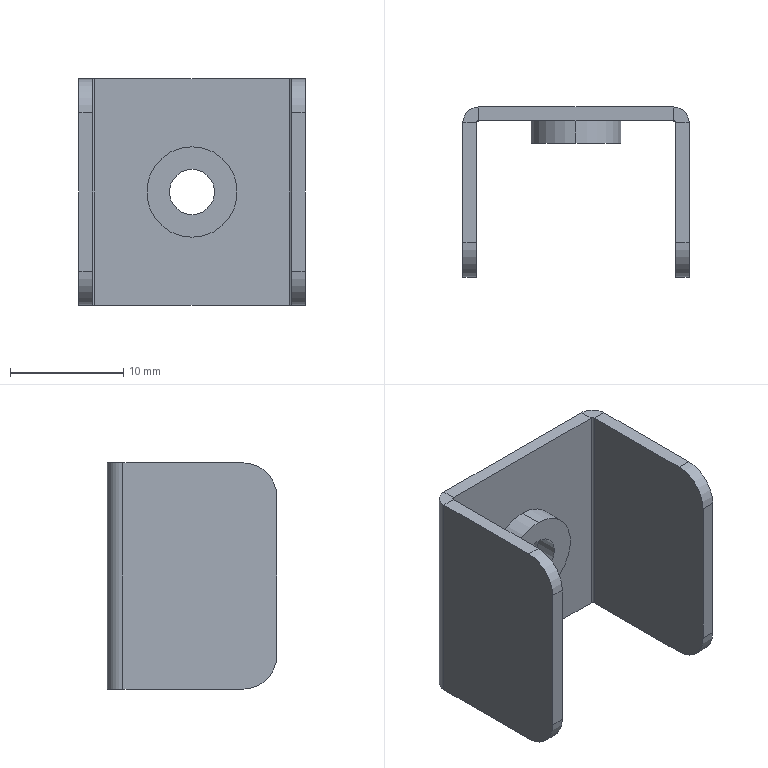Part | SolidWorks | features BaseBody 1 | 1 solid | 34 faces | box 20 x 15 x 20 mm | volume 1173 mm3 | plane 20 | cylinder 14 | commonest cylinder face diameters 6 x4 0.4 x2 2.8 x2 4 x2 4.5 x2 8 x2
STEP:
#1=CARTESIAN_POINT('',(0.,-3.2,-2.));
#2=VERTEX_POINT('',#1);
#3=CARTESIAN_POINT('',(0.,-1.2,-2.));
#4=VERTEX_POINT('',#3);
#5=CARTESIAN_POINT('',(0.,-3.2,-2.));
#6=DIRECTION('',(0.,1.,0.));
#7=VECTOR('',#6,1000.);
#8=LINE('',#5,#7);
#9=EDGE_CURVE('',#2,#4,#8,.T.);
#10=ORIENTED_EDGE('',*,*,#9,.F.);
#11=CARTESIAN_POINT('',(0.,-3.2,2.));
#12=VERTEX_POINT('',#11);
#13=CARTESIAN_POINT('',(0.,-3.2,0.));
#14=DIRECTION('',(0.,-1.,0.));
#15=DIRECTION('',(0.,0.,-1.));
#16=AXIS2_PLACEMENT_3D('',#13,#14,#15);
#17=CIRCLE('',#16,2.);
#18=EDGE_CURVE('',#2,#12,#17,.T.);
#19=ORIENTED_EDGE('',*,*,#18,.T.);
#20=CARTESIAN_POINT('',(0.,-1.2,2.));
#21=VERTEX_POINT('',#20);
#22=CARTESIAN_POINT('',(0.,-3.2,2.));
#23=DIRECTION('',(0.,1.,0.));
#24=VECTOR('',#23,1000.);
#25=LINE('',#22,#24);
#26=EDGE_CURVE('',#12,#21,#25,.T.);
#27=ORIENTED_EDGE('',*,*,#26,.T.);
#28=CARTESIAN_POINT('',(0.,-1.2,0.));
#29=DIRECTION('',(0.,-1.,0.));
#30=DIRECTION('',(0.,0.,-1.));
#31=AXIS2_PLACEMENT_3D('',#28,#29,#30);
#32=CIRCLE('',#31,2.);
#33=EDGE_CURVE('',#4,#21,#32,.T.);
#34=ORIENTED_EDGE('',*,*,#33,.F.);
#35=EDGE_LOOP('',(#10,#19,#27,#34));
#36=FACE_OUTER_BOUND('',#35,.T.);
#37=CARTESIAN_POINT('',(0.,-3.2,0.));
#38=DIRECTION('',(0.,1.,0.));
#39=DIRECTION('',(0.,0.,1.));
#40=AXIS2_PLACEMENT_3D('',#37,#38,#39);
#41=CYLINDRICAL_SURFACE('',#40,2.);
#42=ADVANCED_FACE('',(#36),#41,.F.);
#43=CARTESIAN_POINT('',(0.,-3.2,-4.));
#44=VERTEX_POINT('',#43);
#45=CARTESIAN_POINT('',(0.,-1.2,-4.));
#46=VERTEX_POINT('',#45);
#47=CARTESIAN_POINT('',(0.,-3.2,-4.));
#48=DIRECTION('',(0.,1.,0.));
#49=VECTOR('',#48,1000.);
#50=LINE('',#47,#49);
#51=EDGE_CURVE('',#44,#46,#50,.T.);
#52=ORIENTED_EDGE('',*,*,#51,.F.);
#53=CARTESIAN_POINT('',(0.,-3.2,4.));
#54=VERTEX_POINT('',#53);
#55=CARTESIAN_POINT('',(0.,-3.2,0.));
#56=DIRECTION('',(0.,-1.,0.));
#57=DIRECTION('',(1.,0.,0.));
#58=AXIS2_PLACEMENT_3D('',#55,#56,#57);
#59=CIRCLE('',#58,4.);
#60=EDGE_CURVE('',#54,#44,#59,.T.);
#61=ORIENTED_EDGE('',*,*,#60,.F.);
#62=CARTESIAN_POINT('',(0.,-1.2,4.));
#63=VERTEX_POINT('',#62);
#64=CARTESIAN_POINT('',(0.,-3.2,4.));
#65=DIRECTION('',(0.,1.,0.));
#66=VECTOR('',#65,1000.);
#67=LINE('',#64,#66);
#68=EDGE_CURVE('',#54,#63,#67,.T.);
#69=ORIENTED_EDGE('',*,*,#68,.T.);
#70=CARTESIAN_POINT('',(0.,-1.2,0.));
#71=DIRECTION('',(0.,-1.,0.));
#72=DIRECTION('',(0.,0.,1.));
#73=AXIS2_PLACEMENT_3D('',#70,#71,#72);
#74=CIRCLE('',#73,4.);
#75=EDGE_CURVE('',#63,#46,#74,.T.);
#76=ORIENTED_EDGE('',*,*,#75,.T.);
#77=EDGE_LOOP('',(#52,#61,#69,#76));
#78=FACE_OUTER_BOUND('',#77,.T.);
#79=CARTESIAN_POINT('',(0.,-3.2,0.));
#80=DIRECTION('',(0.,1.,0.));
#81=DIRECTION('',(0.,0.,1.));
#82=AXIS2_PLACEMENT_3D('',#79,#80,#81);
#83=CYLINDRICAL_SURFACE('',#82,4.);
#84=ADVANCED_FACE('',(#78),#83,.T.);
#85=CARTESIAN_POINT('',(0.,-3.2,0.));
#86=DIRECTION('',(0.,-1.,0.));
#87=DIRECTION('',(0.,0.,-1.));
#88=AXIS2_PLACEMENT_3D('',#85,#86,#87);
#89=CIRCLE('',#88,2.);
#90=EDGE_CURVE('',#12,#2,#89,.T.);
#91=ORIENTED_EDGE('',*,*,#90,.F.);
#92=ORIENTED_EDGE('',*,*,#18,.F.);
#93=EDGE_LOOP('',(#91,#92));
#94=FACE_BOUND('',#93,.T.);
#95=ORIENTED_EDGE('',*,*,#60,.T.);
#96=CARTESIAN_POINT('',(0.,-3.2,0.));
#97=DIRECTION('',(0.,-1.,0.));
#98=DIRECTION('',(1.,0.,0.));
#99=AXIS2_PLACEMENT_3D('',#96,#97,#98);
#100=CIRCLE('',#99,4.);
#101=EDGE_CURVE('',#44,#54,#100,.T.);
#102=ORIENTED_EDGE('',*,*,#101,.T.);
#103=EDGE_LOOP('',(#95,#102));
#104=FACE_OUTER_BOUND('',#103,.T.);
#105=CARTESIAN_POINT('',(0.,-3.2,0.));
#106=DIRECTION('',(0.,-1.,0.));
#107=DIRECTION('',(0.,0.,-1.));
#108=AXIS2_PLACEMENT_3D('',#105,#106,#107);
#109=PLANE('',#108);
#110=ADVANCED_FACE('',(#94,#104),#109,.T.);
#111=CARTESIAN_POINT('',(0.,-1.2,0.));
#112=DIRECTION('',(0.,-1.,0.));
#113=DIRECTION('',(0.,0.,-1.));
#114=AXIS2_PLACEMENT_3D('',#111,#112,#113);
#115=CIRCLE('',#114,2.);
#116=EDGE_CURVE('',#21,#4,#115,.T.);
#117=ORIENTED_EDGE('',*,*,#116,.T.);
#118=ORIENTED_EDGE('',*,*,#33,.T.);
#119=EDGE_LOOP('',(#117,#118));
#120=FACE_BOUND('',#119,.T.);
#121=CARTESIAN_POINT('',(0.,-1.2,2.25));
#122=VERTEX_POINT('',#121);
#123=CARTESIAN_POINT('',(0.,-1.2,-2.25));
#124=VERTEX_POINT('',#123);
#125=CARTESIAN_POINT('',(0.,-1.2,0.));
#126=DIRECTION('',(0.,1.,0.));
#127=DIRECTION('',(0.,0.,1.));
#128=AXIS2_PLACEMENT_3D('',#125,#126,#127);
#129=CIRCLE('',#128,2.25);
#130=EDGE_CURVE('',#122,#124,#129,.T.);
#131=ORIENTED_EDGE('',*,*,#130,.T.);
#132=CARTESIAN_POINT('',(0.,-1.2,0.));
#133=DIRECTION('',(0.,1.,0.));
#134=DIRECTION('',(0.,0.,1.));
#135=AXIS2_PLACEMENT_3D('',#132,#133,#134);
#136=CIRCLE('',#135,2.25);
#137=EDGE_CURVE('',#124,#122,#136,.T.);
#138=ORIENTED_EDGE('',*,*,#137,.T.);
#139=EDGE_LOOP('',(#131,#138));
#140=FACE_OUTER_BOUND('',#139,.T.);
#141=CARTESIAN_POINT('',(0.,-1.2,0.));
#142=DIRECTION('',(0.,-1.,0.));
#143=DIRECTION('',(0.,0.,-1.));
#144=AXIS2_PLACEMENT_3D('',#141,#142,#143);
#145=PLANE('',#144);
#146=ADVANCED_FACE('',(#120,#140),#145,.F.);
#147=CARTESIAN_POINT('',(0.,0.,-2.25));
#148=VERTEX_POINT('',#147);
#149=CARTESIAN_POINT('',(0.,-10.,-2.25));
#150=DIRECTION('',(0.,1.,0.));
#151=VECTOR('',#150,1000.);
#152=LINE('',#149,#151);
#153=EDGE_CURVE('',#124,#148,#152,.T.);
#154=ORIENTED_EDGE('',*,*,#153,.F.);
#155=ORIENTED_EDGE('',*,*,#130,.F.);
#156=CARTESIAN_POINT('',(0.,0.,2.25));
#157=VERTEX_POINT('',#156);
#158=CARTESIAN_POINT('',(0.,-10.,2.25));
#159=DIRECTION('',(0.,1.,0.));
#160=VECTOR('',#159,1000.);
#161=LINE('',#158,#160);
#162=EDGE_CURVE('',#122,#157,#161,.T.);
#163=ORIENTED_EDGE('',*,*,#162,.T.);
#164=CARTESIAN_POINT('',(0.,0.,0.));
#165=DIRECTION('',(0.,1.,0.));
#166=DIRECTION('',(0.,0.,1.));
#167=AXIS2_PLACEMENT_3D('',#164,#165,#166);
#168=CIRCLE('',#167,2.25);
#169=EDGE_CURVE('',#157,#148,#168,.T.);
#170=ORIENTED_EDGE('',*,*,#169,.T.);
#171=EDGE_LOOP('',(#154,#155,#163,#170));
#172=FACE_OUTER_BOUND('',#171,.T.);
#173=CARTESIAN_POINT('',(0.,-10.,0.));
#174=DIRECTION('',(0.,1.,0.));
#175=DIRECTION('',(0.,0.,1.));
#176=AXIS2_PLACEMENT_3D('',#173,#174,#175);
#177=CYLINDRICAL_SURFACE('',#176,2.25);
#178=ADVANCED_FACE('',(#172),#177,.F.);
#179=CARTESIAN_POINT('',(10.,-12.,10.));
#180=VERTEX_POINT('',#179);
#181=CARTESIAN_POINT('',(10.,-15.,7.));
#182=VERTEX_POINT('',#181);
#183=CARTESIAN_POINT('',(10.,-12.,7.));
#184=DIRECTION('',(1.,0.,0.));
#185=DIRECTION('',(0.,1.,0.));
#186=AXIS2_PLACEMENT_3D('',#183,#184,#185);
#187=CIRCLE('',#186,3.);
#188=EDGE_CURVE('',#180,#182,#187,.T.);
#189=ORIENTED_EDGE('',*,*,#188,.F.);
#190=CARTESIAN_POINT('',(8.8,-12.,10.));
#191=VERTEX_POINT('',#190);
#192=CARTESIAN_POINT('',(10.,-12.,10.));
#193=DIRECTION('',(1.,0.,0.));
#194=VECTOR('',#193,1000.);
#195=LINE('',#192,#194);
#196=EDGE_CURVE('',#191,#180,#195,.T.);
#197=ORIENTED_EDGE('',*,*,#196,.F.);
#198=CARTESIAN_POINT('',(8.8,-15.,7.));
#199=VERTEX_POINT('',#198);
#200=CARTESIAN_POINT('',(8.8,-12.,7.));
#201=DIRECTION('',(-1.,0.,0.));
#202=DIRECTION('',(0.,1.,0.));
#203=AXIS2_PLACEMENT_3D('',#200,#201,#202);
#204=CIRCLE('',#203,3.);
#205=EDGE_CURVE('',#199,#191,#204,.T.);
#206=ORIENTED_EDGE('',*,*,#205,.F.);
#207=CARTESIAN_POINT('',(10.,-15.,7.));
#208=DIRECTION('',(-1.,0.,0.));
#209=VECTOR('',#208,1000.);
#210=LINE('',#207,#209);
#211=EDGE_CURVE('',#182,#199,#210,.T.);
#212=ORIENTED_EDGE('',*,*,#211,.F.);
#213=EDGE_LOOP('',(#189,#197,#206,#212));
#214=FACE_OUTER_BOUND('',#213,.T.);
#215=CARTESIAN_POINT('',(10.,-12.,7.));
#216=DIRECTION('',(-1.,0.,0.));
#217=DIRECTION('',(0.,-1.,0.));
#218=AXIS2_PLACEMENT_3D('',#215,#216,#217);
#219=CYLINDRICAL_SURFACE('',#218,3.);
#220=ADVANCED_FACE('',(#214),#219,.T.);
#221=CARTESIAN_POINT('',(10.,-15.,-7.));
#222=VERTEX_POINT('',#221);
#223=CARTESIAN_POINT('',(10.,-12.,-10.));
#224=VERTEX_POINT('',#223);
#225=CARTESIAN_POINT('',(10.,-12.,-7.));
#226=DIRECTION('',(1.,0.,0.));
#227=DIRECTION('',(0.,1.,0.));
#228=AXIS2_PLACEMENT_3D('',#225,#226,#227);
#229=CIRCLE('',#228,3.);
#230=EDGE_CURVE('',#222,#224,#229,.T.);
#231=ORIENTED_EDGE('',*,*,#230,.F.);
#232=CARTESIAN_POINT('',(8.8,-15.,-7.));
#233=VERTEX_POINT('',#232);
#234=CARTESIAN_POINT('',(10.,-15.,-7.));
#235=DIRECTION('',(1.,0.,0.));
#236=VECTOR('',#235,1000.);
#237=LINE('',#234,#236);
#238=EDGE_CURVE('',#233,#222,#237,.T.);
#239=ORIENTED_EDGE('',*,*,#238,.F.);
#240=CARTESIAN_POINT('',(8.8,-12.,-10.));
#241=VERTEX_POINT('',#240);
#242=CARTESIAN_POINT('',(8.8,-12.,-7.));
#243=DIRECTION('',(-1.,0.,0.));
#244=DIRECTION('',(0.,1.,0.));
#245=AXIS2_PLACEMENT_3D('',#242,#243,#244);
#246=CIRCLE('',#245,3.);
#247=EDGE_CURVE('',#241,#233,#246,.T.);
#248=ORIENTED_EDGE('',*,*,#247,.F.);
#249=CARTESIAN_POINT('',(10.,-12.,-10.));
#250=DIRECTION('',(-1.,0.,0.));
#251=VECTOR('',#250,1000.);
#252=LINE('',#249,#251);
#253=EDGE_CURVE('',#224,#241,#252,.T.);
#254=ORIENTED_EDGE('',*,*,#253,.F.);
#255=EDGE_LOOP('',(#231,#239,#248,#254));
#256=FACE_OUTER_BOUND('',#255,.T.);
#257=CARTESIAN_POINT('',(10.,-12.,-7.));
#258=DIRECTION('',(-1.,0.,0.));
#259=DIRECTION('',(0.,-1.,0.));
#260=AXIS2_PLACEMENT_3D('',#257,#258,#259);
#261=CYLINDRICAL_SURFACE('',#260,3.);
#262=ADVANCED_FACE('',(#256),#261,.T.);
#263=CARTESIAN_POINT('',(-10.,-12.,-10.));
#264=VERTEX_POINT('',#263);
#265=CARTESIAN_POINT('',(-10.,-15.,-7.));
#266=VERTEX_POINT('',#265);
#267=CARTESIAN_POINT('',(-10.,-12.,-7.));
#268=DIRECTION('',(-1.,0.,0.));
#269=DIRECTION('',(0.,1.,0.));
#270=AXIS2_PLACEMENT_3D('',#267,#268,#269);
#271=CIRCLE('',#270,3.);
#272=EDGE_CURVE('',#264,#266,#271,.T.);
#273=ORIENTED_EDGE('',*,*,#272,.F.);
#274=CARTESIAN_POINT('',(-8.8,-12.,-10.));
#275=VERTEX_POINT('',#274);
#276=CARTESIAN_POINT('',(-10.,-12.,-10.));
#277=DIRECTION('',(-1.,0.,0.));
#278=VECTOR('',#277,1000.);
#279=LINE('',#276,#278);
#280=EDGE_CURVE('',#275,#264,#279,.T.);
#281=ORIENTED_EDGE('',*,*,#280,.F.);
#282=CARTESIAN_POINT('',(-8.8,-15.,-7.));
#283=VERTEX_POINT('',#282);
#284=CARTESIAN_POINT('',(-8.8,-12.,-7.));
#285=DIRECTION('',(1.,0.,0.));
#286=DIRECTION('',(0.,1.,0.));
#287=AXIS2_PLACEMENT_3D('',#284,#285,#286);
#288=CIRCLE('',#287,3.);
#289=EDGE_CURVE('',#283,#275,#288,.T.);
#290=ORIENTED_EDGE('',*,*,#289,.F.);
#291=CARTESIAN_POINT('',(-10.,-15.,-7.));
#292=DIRECTION('',(1.,0.,0.));
#293=VECTOR('',#292,1000.);
#294=LINE('',#291,#293);
#295=EDGE_CURVE('',#266,#283,#294,.T.);
#296=ORIENTED_EDGE('',*,*,#295,.F.);
#297=EDGE_LOOP('',(#273,#281,#290,#296));
#298=FACE_OUTER_BOUND('',#297,.T.);
#299=CARTESIAN_POINT('',(-10.,-12.,-7.));
#300=DIRECTION('',(1.,0.,0.));
#301=DIRECTION('',(0.,1.,0.));
#302=AXIS2_PLACEMENT_3D('',#299,#300,#301);
#303=CYLINDRICAL_SURFACE('',#302,3.);
#304=ADVANCED_FACE('',(#298),#303,.T.);
#305=CARTESIAN_POINT('',(-10.,-15.,7.));
#306=VERTEX_POINT('',#305);
#307=CARTESIAN_POINT('',(-10.,-12.,10.));
#308=VERTEX_POINT('',#307);
#309=CARTESIAN_POINT('',(-10.,-12.,7.));
#310=DIRECTION('',(-1.,0.,0.));
#311=DIRECTION('',(0.,1.,0.));
#312=AXIS2_PLACEMENT_3D('',#309,#310,#311);
#313=CIRCLE('',#312,3.);
#314=EDGE_CURVE('',#306,#308,#313,.T.);
#315=ORIENTED_EDGE('',*,*,#314,.F.);
#316=CARTESIAN_POINT('',(-8.8,-15.,7.));
#317=VERTEX_POINT('',#316);
#318=CARTESIAN_POINT('',(-10.,-15.,7.));
#319=DIRECTION('',(-1.,0.,0.));
#320=VECTOR('',#319,1000.);
#321=LINE('',#318,#320);
#322=EDGE_CURVE('',#317,#306,#321,.T.);
#323=ORIENTED_EDGE('',*,*,#322,.F.);
#324=CARTESIAN_POINT('',(-8.8,-12.,10.));
#325=VERTEX_POINT('',#324);
#326=CARTESIAN_POINT('',(-8.8,-12.,7.));
#327=DIRECTION('',(1.,0.,0.));
#328=DIRECTION('',(0.,1.,0.));
#329=AXIS2_PLACEMENT_3D('',#326,#327,#328);
#330=CIRCLE('',#329,3.);
#331=EDGE_CURVE('',#325,#317,#330,.T.);
#332=ORIENTED_EDGE('',*,*,#331,.F.);
#333=CARTESIAN_POINT('',(-10.,-12.,10.));
#334=DIRECTION('',(1.,0.,0.));
#335=VECTOR('',#334,1000.);
#336=LINE('',#333,#335);
#337=EDGE_CURVE('',#308,#325,#336,.T.);
#338=ORIENTED_EDGE('',*,*,#337,.F.);
#339=EDGE_LOOP('',(#315,#323,#332,#338));
#340=FACE_OUTER_BOUND('',#339,.T.);
#341=CARTESIAN_POINT('',(-10.,-12.,7.));
#342=DIRECTION('',(1.,0.,0.));
#343=DIRECTION('',(0.,1.,0.));
#344=AXIS2_PLACEMENT_3D('',#341,#342,#343);
#345=CYLINDRICAL_SURFACE('',#344,3.);
#346=ADVANCED_FACE('',(#340),#345,.T.);
#347=CARTESIAN_POINT('',(-8.8,-15.,0.));
#348=DIRECTION('',(0.,0.,-1.));
#349=VECTOR('',#348,1000.);
#350=LINE('',#347,#349);
#351=EDGE_CURVE('',#317,#283,#350,.T.);
#352=ORIENTED_EDGE('',*,*,#351,.F.);
#353=ORIENTED_EDGE('',*,*,#322,.T.);
#354=CARTESIAN_POINT('',(-10.,-15.,10.));
#355=DIRECTION('',(0.,0.,-1.));
#356=VECTOR('',#355,1000.);
#357=LINE('',#354,#356);
#358=EDGE_CURVE('',#306,#266,#357,.T.);
#359=ORIENTED_EDGE('',*,*,#358,.T.);
#360=ORIENTED_EDGE('',*,*,#295,.T.);
#361=EDGE_LOOP('',(#352,#353,#359,#360));
#362=FACE_OUTER_BOUND('',#361,.T.);
#363=CARTESIAN_POINT('',(-10.,-15.,10.));
#364=DIRECTION('',(0.,-1.,0.));
#365=DIRECTION('',(-1.,0.,0.));
#366=AXIS2_PLACEMENT_3D('',#363,#364,#365);
#367=PLANE('',#366);
#368=ADVANCED_FACE('',(#362),#367,.T.);
#369=CARTESIAN_POINT('',(-8.8,-1.4,10.));
#370=VERTEX_POINT('',#369);
#371=CARTESIAN_POINT('',(-8.8,0.,10.));
#372=DIRECTION('',(0.,-1.,0.));
#373=VECTOR('',#372,1000.);
#374=LINE('',#371,#373);
#375=EDGE_CURVE('',#370,#325,#374,.T.);
#376=ORIENTED_EDGE('',*,*,#375,.T.);
#377=ORIENTED_EDGE('',*,*,#331,.T.);
#378=ORIENTED_EDGE('',*,*,#351,.T.);
#379=ORIENTED_EDGE('',*,*,#289,.T.);
#380=CARTESIAN_POINT('',(-8.8,-1.4,-10.));
#381=VERTEX_POINT('',#380);
#382=CARTESIAN_POINT('',(-8.8,0.,-10.));
#383=DIRECTION('',(0.,1.,0.));
#384=VECTOR('',#383,1000.);
#385=LINE('',#382,#384);
#386=EDGE_CURVE('',#275,#381,#385,.T.);
#387=ORIENTED_EDGE('',*,*,#386,.T.);
#388=CARTESIAN_POINT('',(-8.8,-1.4,10.));
#389=DIRECTION('',(0.,0.,-1.));
#390=VECTOR('',#389,1000.);
#391=LINE('',#388,#390);
#392=EDGE_CURVE('',#370,#381,#391,.T.);
#393=ORIENTED_EDGE('',*,*,#392,.F.);
#394=EDGE_LOOP('',(#376,#377,#378,#379,#387,#393));
#395=FACE_OUTER_BOUND('',#394,.T.);
#396=CARTESIAN_POINT('',(-8.8,0.,0.));
#397=DIRECTION('',(1.,0.,0.));
#398=DIRECTION('',(0.,-1.,0.));
#399=AXIS2_PLACEMENT_3D('',#396,#397,#398);
#400=PLANE('',#399);
#401=ADVANCED_FACE('',(#395),#400,.T.);
#402=ORIENTED_EDGE('',*,*,#358,.F.);
#403=ORIENTED_EDGE('',*,*,#314,.T.);
#404=CARTESIAN_POINT('',(-10.,-1.4,10.));
#405=VERTEX_POINT('',#404);
#406=CARTESIAN_POINT('',(-10.,-1.2,10.));
#407=DIRECTION('',(0.,-1.,0.));
#408=VECTOR('',#407,1000.);
#409=LINE('',#406,#408);
#410=EDGE_CURVE('',#405,#308,#409,.T.);
#411=ORIENTED_EDGE('',*,*,#410,.F.);
#412=CARTESIAN_POINT('',(-10.,-1.4,-10.));
#413=VERTEX_POINT('',#412);
#414=CARTESIAN_POINT('',(-10.,-1.4,10.));
#415=DIRECTION('',(0.,0.,1.));
#416=VECTOR('',#415,1000.);
#417=LINE('',#414,#416);
#418=EDGE_CURVE('',#413,#405,#417,.T.);
#419=ORIENTED_EDGE('',*,*,#418,.F.);
#420=CARTESIAN_POINT('',(-10.,-15.,-10.));
#421=DIRECTION('',(0.,1.,0.));
#422=VECTOR('',#421,1000.);
#423=LINE('',#420,#422);
#424=EDGE_CURVE('',#264,#413,#423,.T.);
#425=ORIENTED_EDGE('',*,*,#424,.F.);
#426=ORIENTED_EDGE('',*,*,#272,.T.);
#427=EDGE_LOOP('',(#402,#403,#411,#419,#425,#426));
#428=FACE_OUTER_BOUND('',#427,.T.);
#429=CARTESIAN_POINT('',(-10.,0.,0.));
#430=DIRECTION('',(1.,0.,0.));
#431=DIRECTION('',(0.,-1.,0.));
#432=AXIS2_PLACEMENT_3D('',#429,#430,#431);
#433=PLANE('',#432);
#434=ADVANCED_FACE('',(#428),#433,.F.);
#435=ORIENTED_EDGE('',*,*,#386,.F.);
#436=ORIENTED_EDGE('',*,*,#280,.T.);
#437=ORIENTED_EDGE('',*,*,#424,.T.);
#438=CARTESIAN_POINT('',(-8.8,-1.4,-10.));
#439=DIRECTION('',(-1.,0.,0.));
#440=VECTOR('',#439,1000.);
#441=LINE('',#438,#440);
#442=EDGE_CURVE('',#381,#413,#441,.T.);
#443=ORIENTED_EDGE('',*,*,#442,.F.);
#444=EDGE_LOOP('',(#435,#436,#437,#443));
#445=FACE_OUTER_BOUND('',#444,.T.);
#446=CARTESIAN_POINT('',(-10.,-15.,-10.));
#447=DIRECTION('',(0.,0.,-1.));
#448=DIRECTION('',(-1.,0.,0.));
#449=AXIS2_PLACEMENT_3D('',#446,#447,#448);
#450=PLANE('',#449);
#451=ADVANCED_FACE('',(#445),#450,.T.);
#452=ORIENTED_EDGE('',*,*,#410,.T.);
#453=ORIENTED_EDGE('',*,*,#337,.T.);
#454=ORIENTED_EDGE('',*,*,#375,.F.);
#455=CARTESIAN_POINT('',(-10.,-1.4,10.));
#456=DIRECTION('',(-1.,0.,0.));
#457=VECTOR('',#456,1000.);
#458=LINE('',#455,#457);
#459=EDGE_CURVE('',#370,#405,#458,.T.);
#460=ORIENTED_EDGE('',*,*,#459,.T.);
#461=EDGE_LOOP('',(#452,#453,#454,#460));
#462=FACE_OUTER_BOUND('',#461,.T.);
#463=CARTESIAN_POINT('',(-10.,-1.2,10.));
#464=DIRECTION('',(0.,0.,1.));
#465=DIRECTION('',(0.,-1.,0.));
#466=AXIS2_PLACEMENT_3D('',#463,#464,#465);
#467=PLANE('',#466);
#468=ADVANCED_FACE('',(#462),#467,.T.);
#469=CARTESIAN_POINT('',(-8.6,-1.2,-10.));
#470=VERTEX_POINT('',#469);
#471=CARTESIAN_POINT('',(-8.6,-1.2,10.));
#472=VERTEX_POINT('',#471);
#473=CARTESIAN_POINT('',(-8.6,-1.2,-10.));
#474=DIRECTION('',(0.,0.,1.));
#475=VECTOR('',#474,1000.);
#476=LINE('',#473,#475);
#477=EDGE_CURVE('',#470,#472,#476,.T.);
#478=ORIENTED_EDGE('',*,*,#477,.T.);
#479=CARTESIAN_POINT('',(-8.6,-1.4,10.));
#480=DIRECTION('',(0.,0.,1.));
#481=DIRECTION('',(-1.,0.,0.));
#482=AXIS2_PLACEMENT_3D('',#479,#480,#481);
#483=CIRCLE('',#482,0.2);
#484=EDGE_CURVE('',#472,#370,#483,.T.);
#485=ORIENTED_EDGE('',*,*,#484,.T.);
#486=ORIENTED_EDGE('',*,*,#392,.T.);
#487=CARTESIAN_POINT('',(-8.6,-1.4,-10.));
#488=DIRECTION('',(0.,0.,-1.));
#489=DIRECTION('',(-1.,0.,0.));
#490=AXIS2_PLACEMENT_3D('',#487,#488,#489);
#491=CIRCLE('',#490,0.2);
#492=EDGE_CURVE('',#381,#470,#491,.T.);
#493=ORIENTED_EDGE('',*,*,#492,.T.);
#494=EDGE_LOOP('',(#478,#485,#486,#493));
#495=FACE_OUTER_BOUND('',#494,.T.);
#496=CARTESIAN_POINT('',(-8.6,-1.4,-10.));
#497=DIRECTION('',(0.,0.,-1.));
#498=DIRECTION('',(-1.,0.,0.));
#499=AXIS2_PLACEMENT_3D('',#496,#497,#498);
#500=CYLINDRICAL_SURFACE('',#499,0.2);
#501=ADVANCED_FACE('',(#495),#500,.F.);
#502=CARTESIAN_POINT('',(-8.6,0.,-10.));
#503=VERTEX_POINT('',#502);
#504=CARTESIAN_POINT('',(-8.6,0.,10.));
#505=VERTEX_POINT('',#504);
#506=CARTESIAN_POINT('',(-8.6,0.,-10.));
#507=DIRECTION('',(0.,0.,1.));
#508=VECTOR('',#507,1000.);
#509=LINE('',#506,#508);
#510=EDGE_CURVE('',#503,#505,#509,.T.);
#511=ORIENTED_EDGE('',*,*,#510,.F.);
#512=CARTESIAN_POINT('',(-8.6,-1.4,-10.));
#513=DIRECTION('',(0.,0.,-1.));
#514=DIRECTION('',(-1.,0.,0.));
#515=AXIS2_PLACEMENT_3D('',#512,#513,#514);
#516=CIRCLE('',#515,1.4);
#517=EDGE_CURVE('',#413,#503,#516,.T.);
#518=ORIENTED_EDGE('',*,*,#517,.F.);
#519=ORIENTED_EDGE('',*,*,#418,.T.);
#520=CARTESIAN_POINT('',(-8.6,-1.4,10.));
#521=DIRECTION('',(0.,0.,1.));
#522=DIRECTION('',(-1.,0.,0.));
#523=AXIS2_PLACEMENT_3D('',#520,#521,#522);
#524=CIRCLE('',#523,1.4);
#525=EDGE_CURVE('',#505,#405,#524,.T.);
#526=ORIENTED_EDGE('',*,*,#525,.F.);
#527=EDGE_LOOP('',(#511,#518,#519,#526));
#528=FACE_OUTER_BOUND('',#527,.T.);
#529=CARTESIAN_POINT('',(-8.6,-1.4,-10.));
#530=DIRECTION('',(0.,0.,-1.));
#531=DIRECTION('',(-1.,0.,0.));
#532=AXIS2_PLACEMENT_3D('',#529,#530,#531);
#533=CYLINDRICAL_SURFACE('',#532,1.4);
#534=ADVANCED_FACE('',(#528),#533,.T.);
#535=ORIENTED_EDGE('',*,*,#492,.F.);
#536=ORIENTED_EDGE('',*,*,#442,.T.);
#537=ORIENTED_EDGE('',*,*,#517,.T.);
#538=CARTESIAN_POINT('',(-8.6,-1.2,-10.));
#539=DIRECTION('',(0.,1.,0.));
#540=VECTOR('',#539,1000.);
#541=LINE('',#538,#540);
#542=EDGE_CURVE('',#470,#503,#541,.T.);
#543=ORIENTED_EDGE('',*,*,#542,.F.);
#544=EDGE_LOOP('',(#535,#536,#537,#543));
#545=FACE_OUTER_BOUND('',#544,.T.);
#546=CARTESIAN_POINT('',(-8.6,-1.4,-10.));
#547=DIRECTION('',(0.,0.,1.));
#548=DIRECTION('',(1.,0.,0.));
#549=AXIS2_PLACEMENT_3D('',#546,#547,#548);
#550=PLANE('',#549);
#551=ADVANCED_FACE('',(#545),#550,.F.);
#552=ORIENTED_EDGE('',*,*,#459,.F.);
#553=ORIENTED_EDGE('',*,*,#484,.F.);
#554=CARTESIAN_POINT('',(-8.6,-1.2,10.));
#555=DIRECTION('',(0.,1.,0.));
#556=VECTOR('',#555,1000.);
#557=LINE('',#554,#556);
#558=EDGE_CURVE('',#472,#505,#557,.T.);
#559=ORIENTED_EDGE('',*,*,#558,.T.);
#560=ORIENTED_EDGE('',*,*,#525,.T.);
#561=EDGE_LOOP('',(#552,#553,#559,#560));
#562=FACE_OUTER_BOUND('',#561,.T.);
#563=CARTESIAN_POINT('',(-8.6,-1.4,10.));
#564=DIRECTION('',(0.,0.,1.));
#565=DIRECTION('',(1.,0.,0.));
#566=AXIS2_PLACEMENT_3D('',#563,#564,#565);
#567=PLANE('',#566);
#568=ADVANCED_FACE('',(#562),#567,.T.);
#569=CARTESIAN_POINT('',(8.8,-15.,0.));
#570=DIRECTION('',(0.,0.,1.));
#571=VECTOR('',#570,1000.);
#572=LINE('',#569,#571);
#573=EDGE_CURVE('',#233,#199,#572,.T.);
#574=ORIENTED_EDGE('',*,*,#573,.F.);
#575=ORIENTED_EDGE('',*,*,#238,.T.);
#576=CARTESIAN_POINT('',(10.,-15.,10.));
#577=DIRECTION('',(0.,0.,1.));
#578=VECTOR('',#577,1000.);
#579=LINE('',#576,#578);
#580=EDGE_CURVE('',#222,#182,#579,.T.);
#581=ORIENTED_EDGE('',*,*,#580,.T.);
#582=ORIENTED_EDGE('',*,*,#211,.T.);
#583=EDGE_LOOP('',(#574,#575,#581,#582));
#584=FACE_OUTER_BOUND('',#583,.T.);
#585=CARTESIAN_POINT('',(10.,-15.,10.));
#586=DIRECTION('',(0.,-1.,0.));
#587=DIRECTION('',(0.,0.,-1.));
#588=AXIS2_PLACEMENT_3D('',#585,#586,#587);
#589=PLANE('',#588);
#590=ADVANCED_FACE('',(#584),#589,.T.);
#591=CARTESIAN_POINT('',(8.8,-1.4,-10.));
#592=VERTEX_POINT('',#591);
#593=CARTESIAN_POINT('',(8.8,0.,-10.));
#594=DIRECTION('',(0.,-1.,0.));
#595=VECTOR('',#594,1000.);
#596=LINE('',#593,#595);
#597=EDGE_CURVE('',#592,#241,#596,.T.);
#598=ORIENTED_EDGE('',*,*,#597,.T.);
#599=ORIENTED_EDGE('',*,*,#247,.T.);
#600=ORIENTED_EDGE('',*,*,#573,.T.);
#601=ORIENTED_EDGE('',*,*,#205,.T.);
#602=CARTESIAN_POINT('',(8.8,-1.4,10.));
#603=VERTEX_POINT('',#602);
#604=CARTESIAN_POINT('',(8.8,0.,10.));
#605=DIRECTION('',(0.,1.,0.));
#606=VECTOR('',#605,1000.);
#607=LINE('',#604,#606);
#608=EDGE_CURVE('',#191,#603,#607,.T.);
#609=ORIENTED_EDGE('',*,*,#608,.T.);
#610=CARTESIAN_POINT('',(8.8,-1.4,-10.));
#611=DIRECTION('',(0.,0.,1.));
#612=VECTOR('',#611,1000.);
#613=LINE('',#610,#612);
#614=EDGE_CURVE('',#592,#603,#613,.T.);
#615=ORIENTED_EDGE('',*,*,#614,.F.);
#616=EDGE_LOOP('',(#598,#599,#600,#601,#609,#615));
#617=FACE_OUTER_BOUND('',#616,.T.);
#618=CARTESIAN_POINT('',(8.8,0.,0.));
#619=DIRECTION('',(1.,0.,0.));
#620=DIRECTION('',(0.,1.,0.));
#621=AXIS2_PLACEMENT_3D('',#618,#619,#620);
#622=PLANE('',#621);
#623=ADVANCED_FACE('',(#617),#622,.F.);
#624=ORIENTED_EDGE('',*,*,#580,.F.);
#625=ORIENTED_EDGE('',*,*,#230,.T.);
#626=CARTESIAN_POINT('',(10.,-1.4,-10.));
#627=VERTEX_POINT('',#626);
#628=CARTESIAN_POINT('',(10.,-15.,-10.));
#629=DIRECTION('',(0.,-1.,0.));
#630=VECTOR('',#629,1000.);
#631=LINE('',#628,#630);
#632=EDGE_CURVE('',#627,#224,#631,.T.);
#633=ORIENTED_EDGE('',*,*,#632,.F.);
#634=CARTESIAN_POINT('',(10.,-1.4,10.));
#635=VERTEX_POINT('',#634);
#636=CARTESIAN_POINT('',(10.,-1.4,0.));
#637=DIRECTION('',(0.,0.,1.));
#638=VECTOR('',#637,1000.);
#639=LINE('',#636,#638);
#640=EDGE_CURVE('',#627,#635,#639,.T.);
#641=ORIENTED_EDGE('',*,*,#640,.T.);
#642=CARTESIAN_POINT('',(10.,-1.2,10.));
#643=DIRECTION('',(0.,1.,0.));
#644=VECTOR('',#643,1000.);
#645=LINE('',#642,#644);
#646=EDGE_CURVE('',#180,#635,#645,.T.);
#647=ORIENTED_EDGE('',*,*,#646,.F.);
#648=ORIENTED_EDGE('',*,*,#188,.T.);
#649=EDGE_LOOP('',(#624,#625,#633,#641,#647,#648));
#650=FACE_OUTER_BOUND('',#649,.T.);
#651=CARTESIAN_POINT('',(10.,0.,0.));
#652=DIRECTION('',(1.,0.,0.));
#653=DIRECTION('',(0.,1.,0.));
#654=AXIS2_PLACEMENT_3D('',#651,#652,#653);
#655=PLANE('',#654);
#656=ADVANCED_FACE('',(#650),#655,.T.);
#657=ORIENTED_EDGE('',*,*,#632,.T.);
#658=ORIENTED_EDGE('',*,*,#253,.T.);
#659=ORIENTED_EDGE('',*,*,#597,.F.);
#660=CARTESIAN_POINT('',(10.,-1.4,-10.));
#661=DIRECTION('',(1.,0.,0.));
#662=VECTOR('',#661,1000.);
#663=LINE('',#660,#662);
#664=EDGE_CURVE('',#592,#627,#663,.T.);
#665=ORIENTED_EDGE('',*,*,#664,.T.);
#666=EDGE_LOOP('',(#657,#658,#659,#665));
#667=FACE_OUTER_BOUND('',#666,.T.);
#668=CARTESIAN_POINT('',(10.,-15.,-10.));
#669=DIRECTION('',(0.,0.,-1.));
#670=DIRECTION('',(0.,-1.,0.));
#671=AXIS2_PLACEMENT_3D('',#668,#669,#670);
#672=PLANE('',#671);
#673=ADVANCED_FACE('',(#667),#672,.T.);
#674=ORIENTED_EDGE('',*,*,#608,.F.);
#675=ORIENTED_EDGE('',*,*,#196,.T.);
#676=ORIENTED_EDGE('',*,*,#646,.T.);
#677=CARTESIAN_POINT('',(8.8,-1.4,10.));
#678=DIRECTION('',(1.,0.,0.));
#679=VECTOR('',#678,1000.);
#680=LINE('',#677,#679);
#681=EDGE_CURVE('',#603,#635,#680,.T.);
#682=ORIENTED_EDGE('',*,*,#681,.F.);
#683=EDGE_LOOP('',(#674,#675,#676,#682));
#684=FACE_OUTER_BOUND('',#683,.T.);
#685=CARTESIAN_POINT('',(10.,-1.2,10.));
#686=DIRECTION('',(0.,0.,1.));
#687=DIRECTION('',(0.,-1.,0.));
#688=AXIS2_PLACEMENT_3D('',#685,#686,#687);
#689=PLANE('',#688);
#690=ADVANCED_FACE('',(#684),#689,.T.);
#691=CARTESIAN_POINT('',(8.6,-1.2,10.));
#692=VERTEX_POINT('',#691);
#693=CARTESIAN_POINT('',(8.6,-1.2,-10.));
#694=VERTEX_POINT('',#693);
#695=CARTESIAN_POINT('',(8.6,-1.2,10.));
#696=DIRECTION('',(0.,0.,-1.));
#697=VECTOR('',#696,1000.);
#698=LINE('',#695,#697);
#699=EDGE_CURVE('',#692,#694,#698,.T.);
#700=ORIENTED_EDGE('',*,*,#699,.T.);
#701=CARTESIAN_POINT('',(8.6,-1.4,-10.));
#702=DIRECTION('',(0.,0.,-1.));
#703=DIRECTION('',(1.,0.,0.));
#704=AXIS2_PLACEMENT_3D('',#701,#702,#703);
#705=CIRCLE('',#704,0.2);
#706=EDGE_CURVE('',#694,#592,#705,.T.);
#707=ORIENTED_EDGE('',*,*,#706,.T.);
#708=ORIENTED_EDGE('',*,*,#614,.T.);
#709=CARTESIAN_POINT('',(8.6,-1.4,10.));
#710=DIRECTION('',(0.,0.,1.));
#711=DIRECTION('',(1.,0.,0.));
#712=AXIS2_PLACEMENT_3D('',#709,#710,#711);
#713=CIRCLE('',#712,0.2);
#714=EDGE_CURVE('',#603,#692,#713,.T.);
#715=ORIENTED_EDGE('',*,*,#714,.T.);
#716=EDGE_LOOP('',(#700,#707,#708,#715));
#717=FACE_OUTER_BOUND('',#716,.T.);
#718=CARTESIAN_POINT('',(8.6,-1.4,10.));
#719=DIRECTION('',(0.,0.,1.));
#720=DIRECTION('',(1.,0.,0.));
#721=AXIS2_PLACEMENT_3D('',#718,#719,#720);
#722=CYLINDRICAL_SURFACE('',#721,0.2);
#723=ADVANCED_FACE('',(#717),#722,.F.);
#724=CARTESIAN_POINT('',(8.6,0.,10.));
#725=VERTEX_POINT('',#724);
#726=CARTESIAN_POINT('',(8.6,0.,-10.));
#727=VERTEX_POINT('',#726);
#728=CARTESIAN_POINT('',(8.6,0.,10.));
#729=DIRECTION('',(0.,0.,-1.));
#730=VECTOR('',#729,1000.);
#731=LINE('',#728,#730);
#732=EDGE_CURVE('',#725,#727,#731,.T.);
#733=ORIENTED_EDGE('',*,*,#732,.F.);
#734=CARTESIAN_POINT('',(8.6,-1.4,10.));
#735=DIRECTION('',(0.,0.,1.));
#736=DIRECTION('',(1.,0.,0.));
#737=AXIS2_PLACEMENT_3D('',#734,#735,#736);
#738=CIRCLE('',#737,1.4);
#739=EDGE_CURVE('',#635,#725,#738,.T.);
#740=ORIENTED_EDGE('',*,*,#739,.F.);
#741=ORIENTED_EDGE('',*,*,#640,.F.);
#742=CARTESIAN_POINT('',(8.6,-1.4,-10.));
#743=DIRECTION('',(0.,0.,-1.));
#744=DIRECTION('',(1.,0.,0.));
#745=AXIS2_PLACEMENT_3D('',#742,#743,#744);
#746=CIRCLE('',#745,1.4);
#747=EDGE_CURVE('',#727,#627,#746,.T.);
#748=ORIENTED_EDGE('',*,*,#747,.F.);
#749=EDGE_LOOP('',(#733,#740,#741,#748));
#750=FACE_OUTER_BOUND('',#749,.T.);
#751=CARTESIAN_POINT('',(8.6,-1.4,10.));
#752=DIRECTION('',(0.,0.,1.));
#753=DIRECTION('',(1.,0.,0.));
#754=AXIS2_PLACEMENT_3D('',#751,#752,#753);
#755=CYLINDRICAL_SURFACE('',#754,1.4);
#756=ADVANCED_FACE('',(#750),#755,.T.);
#757=ORIENTED_EDGE('',*,*,#714,.F.);
#758=ORIENTED_EDGE('',*,*,#681,.T.);
#759=ORIENTED_EDGE('',*,*,#739,.T.);
#760=CARTESIAN_POINT('',(8.6,-1.2,10.));
#761=DIRECTION('',(0.,1.,0.));
#762=VECTOR('',#761,1000.);
#763=LINE('',#760,#762);
#764=EDGE_CURVE('',#692,#725,#763,.T.);
#765=ORIENTED_EDGE('',*,*,#764,.F.);
#766=EDGE_LOOP('',(#757,#758,#759,#765));
#767=FACE_OUTER_BOUND('',#766,.T.);
#768=CARTESIAN_POINT('',(8.6,-1.4,10.));
#769=DIRECTION('',(0.,0.,-1.));
#770=DIRECTION('',(0.,-1.,0.));
#771=AXIS2_PLACEMENT_3D('',#768,#769,#770);
#772=PLANE('',#771);
#773=ADVANCED_FACE('',(#767),#772,.F.);
#774=ORIENTED_EDGE('',*,*,#664,.F.);
#775=ORIENTED_EDGE('',*,*,#706,.F.);
#776=CARTESIAN_POINT('',(8.6,-1.2,-10.));
#777=DIRECTION('',(0.,1.,0.));
#778=VECTOR('',#777,1000.);
#779=LINE('',#776,#778);
#780=EDGE_CURVE('',#694,#727,#779,.T.);
#781=ORIENTED_EDGE('',*,*,#780,.T.);
#782=ORIENTED_EDGE('',*,*,#747,.T.);
#783=EDGE_LOOP('',(#774,#775,#781,#782));
#784=FACE_OUTER_BOUND('',#783,.T.);
#785=CARTESIAN_POINT('',(8.6,-1.4,-10.));
#786=DIRECTION('',(0.,0.,-1.));
#787=DIRECTION('',(0.,-1.,0.));
#788=AXIS2_PLACEMENT_3D('',#785,#786,#787);
#789=PLANE('',#788);
#790=ADVANCED_FACE('',(#784),#789,.T.);
#791=ORIENTED_EDGE('',*,*,#558,.F.);
#792=CARTESIAN_POINT('',(-10.,-1.2,10.));
#793=DIRECTION('',(1.,0.,0.));
#794=VECTOR('',#793,1000.);
#795=LINE('',#792,#794);
#796=EDGE_CURVE('',#472,#692,#795,.T.);
#797=ORIENTED_EDGE('',*,*,#796,.T.);
#798=ORIENTED_EDGE('',*,*,#764,.T.);
#799=CARTESIAN_POINT('',(-10.,0.,10.));
#800=DIRECTION('',(1.,0.,0.));
#801=VECTOR('',#800,1000.);
#802=LINE('',#799,#801);
#803=EDGE_CURVE('',#505,#725,#802,.T.);
#804=ORIENTED_EDGE('',*,*,#803,.F.);
#805=EDGE_LOOP('',(#791,#797,#798,#804));
#806=FACE_OUTER_BOUND('',#805,.T.);
#807=CARTESIAN_POINT('',(-10.,-1.2,10.));
#808=DIRECTION('',(0.,0.,1.));
#809=DIRECTION('',(1.,0.,0.));
#810=AXIS2_PLACEMENT_3D('',#807,#808,#809);
#811=PLANE('',#810);
#812=ADVANCED_FACE('',(#806),#811,.T.);
#813=CARTESIAN_POINT('',(-10.,-1.2,-10.));
#814=DIRECTION('',(-1.,0.,0.));
#815=VECTOR('',#814,1000.);
#816=LINE('',#813,#815);
#817=EDGE_CURVE('',#694,#470,#816,.T.);
#818=ORIENTED_EDGE('',*,*,#817,.T.);
#819=ORIENTED_EDGE('',*,*,#542,.T.);
#820=CARTESIAN_POINT('',(-10.,0.,-10.));
#821=DIRECTION('',(-1.,0.,0.));
#822=VECTOR('',#821,1000.);
#823=LINE('',#820,#822);
#824=EDGE_CURVE('',#727,#503,#823,.T.);
#825=ORIENTED_EDGE('',*,*,#824,.F.);
#826=ORIENTED_EDGE('',*,*,#780,.F.);
#827=EDGE_LOOP('',(#818,#819,#825,#826));
#828=FACE_OUTER_BOUND('',#827,.T.);
#829=CARTESIAN_POINT('',(-10.,-1.2,-10.));
#830=DIRECTION('',(0.,0.,-1.));
#831=DIRECTION('',(0.,-1.,0.));
#832=AXIS2_PLACEMENT_3D('',#829,#830,#831);
#833=PLANE('',#832);
#834=ADVANCED_FACE('',(#828),#833,.T.);
#835=ORIENTED_EDGE('',*,*,#169,.F.);
#836=CARTESIAN_POINT('',(0.,0.,0.));
#837=DIRECTION('',(0.,1.,0.));
#838=DIRECTION('',(0.,0.,1.));
#839=AXIS2_PLACEMENT_3D('',#836,#837,#838);
#840=CIRCLE('',#839,2.25);
#841=EDGE_CURVE('',#148,#157,#840,.T.);
#842=ORIENTED_EDGE('',*,*,#841,.F.);
#843=EDGE_LOOP('',(#835,#842));
#844=FACE_BOUND('',#843,.T.);
#845=ORIENTED_EDGE('',*,*,#824,.T.);
#846=ORIENTED_EDGE('',*,*,#510,.T.);
#847=ORIENTED_EDGE('',*,*,#803,.T.);
#848=ORIENTED_EDGE('',*,*,#732,.T.);
#849=EDGE_LOOP('',(#845,#846,#847,#848));
#850=FACE_OUTER_BOUND('',#849,.T.);
#851=CARTESIAN_POINT('',(0.,0.,0.));
#852=DIRECTION('',(0.,1.,0.));
#853=DIRECTION('',(1.,0.,0.));
#854=AXIS2_PLACEMENT_3D('',#851,#852,#853);
#855=PLANE('',#854);
#856=ADVANCED_FACE('',(#844,#850),#855,.T.);
#857=ORIENTED_EDGE('',*,*,#75,.F.);
#858=CARTESIAN_POINT('',(0.,-1.2,0.));
#859=DIRECTION('',(0.,-1.,0.));
#860=DIRECTION('',(0.,0.,1.));
#861=AXIS2_PLACEMENT_3D('',#858,#859,#860);
#862=CIRCLE('',#861,4.);
#863=EDGE_CURVE('',#46,#63,#862,.T.);
#864=ORIENTED_EDGE('',*,*,#863,.F.);
#865=EDGE_LOOP('',(#857,#864));
#866=FACE_BOUND('',#865,.T.);
#867=ORIENTED_EDGE('',*,*,#477,.F.);
#868=ORIENTED_EDGE('',*,*,#817,.F.);
#869=ORIENTED_EDGE('',*,*,#699,.F.);
#870=ORIENTED_EDGE('',*,*,#796,.F.);
#871=EDGE_LOOP('',(#867,#868,#869,#870));
#872=FACE_OUTER_BOUND('',#871,.T.);
#873=CARTESIAN_POINT('',(0.,-1.2,0.));
#874=DIRECTION('',(0.,1.,0.));
#875=DIRECTION('',(1.,0.,0.));
#876=AXIS2_PLACEMENT_3D('',#873,#874,#875);
#877=PLANE('',#876);
#878=ADVANCED_FACE('',(#866,#872),#877,.F.);
#879=ORIENTED_EDGE('',*,*,#137,.F.);
#880=ORIENTED_EDGE('',*,*,#153,.T.);
#881=ORIENTED_EDGE('',*,*,#841,.T.);
#882=ORIENTED_EDGE('',*,*,#162,.F.);
#883=EDGE_LOOP('',(#879,#880,#881,#882));
#884=FACE_OUTER_BOUND('',#883,.T.);
#885=CARTESIAN_POINT('',(0.,-10.,0.));
#886=DIRECTION('',(0.,1.,0.));
#887=DIRECTION('',(0.,0.,1.));
#888=AXIS2_PLACEMENT_3D('',#885,#886,#887);
#889=CYLINDRICAL_SURFACE('',#888,2.25);
#890=ADVANCED_FACE('',(#884),#889,.F.);
#891=ORIENTED_EDGE('',*,*,#101,.F.);
#892=ORIENTED_EDGE('',*,*,#51,.T.);
#893=ORIENTED_EDGE('',*,*,#863,.T.);
#894=ORIENTED_EDGE('',*,*,#68,.F.);
#895=EDGE_LOOP('',(#891,#892,#893,#894));
#896=FACE_OUTER_BOUND('',#895,.T.);
#897=CARTESIAN_POINT('',(0.,-3.2,0.));
#898=DIRECTION('',(0.,1.,0.));
#899=DIRECTION('',(0.,0.,1.));
#900=AXIS2_PLACEMENT_3D('',#897,#898,#899);
#901=CYLINDRICAL_SURFACE('',#900,4.);
#902=ADVANCED_FACE('',(#896),#901,.T.);
#903=ORIENTED_EDGE('',*,*,#90,.T.);
#904=ORIENTED_EDGE('',*,*,#9,.T.);
#905=ORIENTED_EDGE('',*,*,#116,.F.);
#906=ORIENTED_EDGE('',*,*,#26,.F.);
#907=EDGE_LOOP('',(#903,#904,#905,#906));
#908=FACE_OUTER_BOUND('',#907,.T.);
#909=CARTESIAN_POINT('',(0.,-3.2,0.));
#910=DIRECTION('',(0.,1.,0.));
#911=DIRECTION('',(0.,0.,1.));
#912=AXIS2_PLACEMENT_3D('',#909,#910,#911);
#913=CYLINDRICAL_SURFACE('',#912,2.);
#914=ADVANCED_FACE('',(#908),#913,.F.);
#915=CLOSED_SHELL('',(#42,#84,#110,#146,#178,#220,#262,#304,#346,#368,#401,#434,#451,#468,#501,#534,#551,#568,#590,#623,#656,#673,#690,#723,#756,#773,#790,#812,#834,#856,#878,#890,#902,#914));
#916=MANIFOLD_SOLID_BREP('',#915);
#917=CARTESIAN_POINT('',(0.,0.,0.));
#918=DIRECTION('',(0.,0.,1.));
#919=DIRECTION('',(1.,0.,0.));
#920=AXIS2_PLACEMENT_3D('',#917,#918,#919);
#921=(LENGTH_UNIT()NAMED_UNIT(*)SI_UNIT(.MILLI.,.METRE.));
#922=UNCERTAINTY_MEASURE_WITH_UNIT(LENGTH_MEASURE(0.00001),#921,'','');
#923=(NAMED_UNIT(*)PLANE_ANGLE_UNIT()SI_UNIT($,.RADIAN.));
#924=(NAMED_UNIT(*)SI_UNIT($,.STERADIAN.)SOLID_ANGLE_UNIT());
#925=(GEOMETRIC_REPRESENTATION_CONTEXT(3)GLOBAL_UNCERTAINTY_ASSIGNED_CONTEXT((#922))GLOBAL_UNIT_ASSIGNED_CONTEXT((#921,#923,#924))REPRESENTATION_CONTEXT('',''));
#926=ADVANCED_BREP_SHAPE_REPRESENTATION('',(#916,#920),#925);